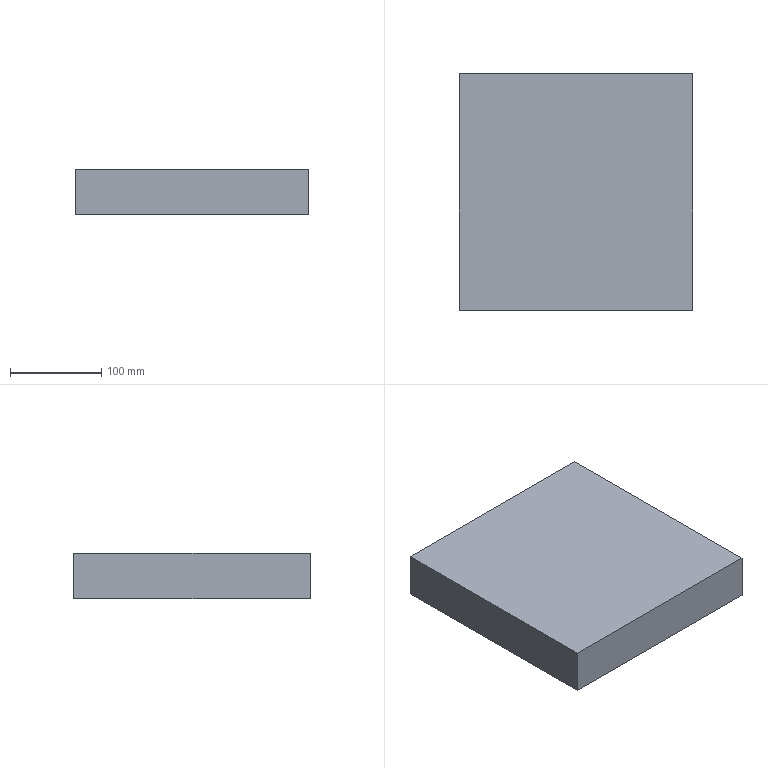Part | STEP file | 1 solid | 6 faces | box 255.311 x 259.164 x 50 mm | volume 3308367 mm3 | plane 6
STEP:
#1=CARTESIAN_POINT('',(0.,0.,0.));
#2=DIRECTION('',(0.,0.,1.));
#3=DIRECTION('',(1.,0.,0.));
#4=AXIS2_PLACEMENT_3D('',#1,#2,#3);
#5=CARTESIAN_POINT('',(-550.,-240.836,393.641));
#6=VERTEX_POINT('',#5);
#7=CARTESIAN_POINT('',(-550.,-500.,393.641));
#8=VERTEX_POINT('',#7);
#9=CARTESIAN_POINT('',(-550.,-240.836,393.641));
#10=DIRECTION('',(0.,-1.,0.));
#11=VECTOR('',#10,1.);
#12=LINE('',#9,#11);
#13=CARTESIAN_POINT('',(-550.,-240.836,343.641));
#14=DIRECTION('',(-1.,0.,0.));
#15=DIRECTION('',(0.,0.,1.));
#16=AXIS2_PLACEMENT_3D('',#13,#14,#15);
#17=PLANE('',#16);
#18=CARTESIAN_POINT('',(50.,0.));
#19=DIRECTION('',(0.,-1.));
#20=VECTOR('',#19,1.);
#21=LINE('',#18,#20);
#22=(GEOMETRIC_REPRESENTATION_CONTEXT(2)PARAMETRIC_REPRESENTATION_CONTEXT()REPRESENTATION_CONTEXT('',''));
#23=DEFINITIONAL_REPRESENTATION('',(#21),#22);
#24=PCURVE('',#17,#23);
#25=CARTESIAN_POINT('',(0.,0.,393.641));
#26=DIRECTION('',(0.,0.,1.));
#27=DIRECTION('',(1.,0.,0.));
#28=AXIS2_PLACEMENT_3D('',#25,#26,#27);
#29=PLANE('',#28);
#30=CARTESIAN_POINT('',(-550.,-240.836));
#31=DIRECTION('',(0.,-1.));
#32=VECTOR('',#31,1.);
#33=LINE('',#30,#32);
#34=(GEOMETRIC_REPRESENTATION_CONTEXT(2)PARAMETRIC_REPRESENTATION_CONTEXT()REPRESENTATION_CONTEXT('',''));
#35=DEFINITIONAL_REPRESENTATION('',(#33),#34);
#36=PCURVE('',#29,#35);
#37=SURFACE_CURVE('',#12,(#24,#36),.PCURVE_S1.);
#38=EDGE_CURVE('',#6,#8,#37,.T.);
#39=ORIENTED_EDGE('',*,*,#38,.F.);
#40=CARTESIAN_POINT('',(-550.,-240.836,343.641));
#41=VERTEX_POINT('',#40);
#42=CARTESIAN_POINT('',(-550.,-240.836,343.641));
#43=DIRECTION('',(0.,0.,1.));
#44=VECTOR('',#43,1.);
#45=LINE('',#42,#44);
#46=CARTESIAN_POINT('',(0.,0.));
#47=DIRECTION('',(1.,0.));
#48=VECTOR('',#47,1.);
#49=LINE('',#46,#48);
#50=(GEOMETRIC_REPRESENTATION_CONTEXT(2)PARAMETRIC_REPRESENTATION_CONTEXT()REPRESENTATION_CONTEXT('',''));
#51=DEFINITIONAL_REPRESENTATION('',(#49),#50);
#52=PCURVE('',#17,#51);
#53=CARTESIAN_POINT('',(-550.,-240.836,343.641));
#54=DIRECTION('',(0.,1.,0.));
#55=DIRECTION('',(0.,0.,1.));
#56=AXIS2_PLACEMENT_3D('',#53,#54,#55);
#57=PLANE('',#56);
#58=CARTESIAN_POINT('',(0.,0.));
#59=DIRECTION('',(1.,0.));
#60=VECTOR('',#59,1.);
#61=LINE('',#58,#60);
#62=(GEOMETRIC_REPRESENTATION_CONTEXT(2)PARAMETRIC_REPRESENTATION_CONTEXT()REPRESENTATION_CONTEXT('',''));
#63=DEFINITIONAL_REPRESENTATION('',(#61),#62);
#64=PCURVE('',#57,#63);
#65=SURFACE_CURVE('',#45,(#52,#64),.PCURVE_S1.);
#66=EDGE_CURVE('',#41,#6,#65,.T.);
#67=ORIENTED_EDGE('',*,*,#66,.F.);
#68=CARTESIAN_POINT('',(-550.,-500.,343.641));
#69=VERTEX_POINT('',#68);
#70=CARTESIAN_POINT('',(-550.,-240.836,343.641));
#71=DIRECTION('',(0.,-1.,0.));
#72=VECTOR('',#71,1.);
#73=LINE('',#70,#72);
#74=CARTESIAN_POINT('',(0.,0.));
#75=DIRECTION('',(0.,-1.));
#76=VECTOR('',#75,1.);
#77=LINE('',#74,#76);
#78=(GEOMETRIC_REPRESENTATION_CONTEXT(2)PARAMETRIC_REPRESENTATION_CONTEXT()REPRESENTATION_CONTEXT('',''));
#79=DEFINITIONAL_REPRESENTATION('',(#77),#78);
#80=PCURVE('',#17,#79);
#81=CARTESIAN_POINT('',(0.,0.,343.641));
#82=DIRECTION('',(0.,0.,1.));
#83=DIRECTION('',(1.,0.,0.));
#84=AXIS2_PLACEMENT_3D('',#81,#82,#83);
#85=PLANE('',#84);
#86=CARTESIAN_POINT('',(-550.,-240.836));
#87=DIRECTION('',(0.,-1.));
#88=VECTOR('',#87,1.);
#89=LINE('',#86,#88);
#90=(GEOMETRIC_REPRESENTATION_CONTEXT(2)PARAMETRIC_REPRESENTATION_CONTEXT()REPRESENTATION_CONTEXT('',''));
#91=DEFINITIONAL_REPRESENTATION('',(#89),#90);
#92=PCURVE('',#85,#91);
#93=SURFACE_CURVE('',#73,(#80,#92),.PCURVE_S1.);
#94=EDGE_CURVE('',#41,#69,#93,.T.);
#95=ORIENTED_EDGE('',*,*,#94,.T.);
#96=CARTESIAN_POINT('',(-550.,-500.,343.641));
#97=DIRECTION('',(0.,0.,1.));
#98=VECTOR('',#97,1.);
#99=LINE('',#96,#98);
#100=CARTESIAN_POINT('',(0.,-259.164));
#101=DIRECTION('',(1.,0.));
#102=VECTOR('',#101,1.);
#103=LINE('',#100,#102);
#104=(GEOMETRIC_REPRESENTATION_CONTEXT(2)PARAMETRIC_REPRESENTATION_CONTEXT()REPRESENTATION_CONTEXT('',''));
#105=DEFINITIONAL_REPRESENTATION('',(#103),#104);
#106=PCURVE('',#17,#105);
#107=CARTESIAN_POINT('',(-550.,-500.,343.641));
#108=DIRECTION('',(0.,-1.,0.));
#109=DIRECTION('',(0.,0.,-1.));
#110=AXIS2_PLACEMENT_3D('',#107,#108,#109);
#111=PLANE('',#110);
#112=CARTESIAN_POINT('',(0.,0.));
#113=DIRECTION('',(-1.,0.));
#114=VECTOR('',#113,1.);
#115=LINE('',#112,#114);
#116=(GEOMETRIC_REPRESENTATION_CONTEXT(2)PARAMETRIC_REPRESENTATION_CONTEXT()REPRESENTATION_CONTEXT('',''));
#117=DEFINITIONAL_REPRESENTATION('',(#115),#116);
#118=PCURVE('',#111,#117);
#119=SURFACE_CURVE('',#99,(#106,#118),.PCURVE_S1.);
#120=EDGE_CURVE('',#69,#8,#119,.T.);
#121=ORIENTED_EDGE('',*,*,#120,.T.);
#122=EDGE_LOOP('',(#39,#67,#95,#121));
#123=FACE_BOUND('',#122,.T.);
#124=ADVANCED_FACE('',(#123),#17,.T.);
#125=CARTESIAN_POINT('',(-294.689,-240.836,393.641));
#126=VERTEX_POINT('',#125);
#127=CARTESIAN_POINT('',(-550.,-240.836,393.641));
#128=DIRECTION('',(-1.,0.,0.));
#129=VECTOR('',#128,1.);
#130=LINE('',#127,#129);
#131=CARTESIAN_POINT('',(50.,0.));
#132=DIRECTION('',(0.,-1.));
#133=VECTOR('',#132,1.);
#134=LINE('',#131,#133);
#135=(GEOMETRIC_REPRESENTATION_CONTEXT(2)PARAMETRIC_REPRESENTATION_CONTEXT()REPRESENTATION_CONTEXT('',''));
#136=DEFINITIONAL_REPRESENTATION('',(#134),#135);
#137=PCURVE('',#57,#136);
#138=CARTESIAN_POINT('',(-550.,-240.836));
#139=DIRECTION('',(-1.,0.));
#140=VECTOR('',#139,1.);
#141=LINE('',#138,#140);
#142=(GEOMETRIC_REPRESENTATION_CONTEXT(2)PARAMETRIC_REPRESENTATION_CONTEXT()REPRESENTATION_CONTEXT('',''));
#143=DEFINITIONAL_REPRESENTATION('',(#141),#142);
#144=PCURVE('',#29,#143);
#145=SURFACE_CURVE('',#130,(#137,#144),.PCURVE_S1.);
#146=EDGE_CURVE('',#126,#6,#145,.T.);
#147=ORIENTED_EDGE('',*,*,#146,.F.);
#148=CARTESIAN_POINT('',(-294.689,-240.836,343.641));
#149=VERTEX_POINT('',#148);
#150=CARTESIAN_POINT('',(-294.689,-240.836,343.641));
#151=DIRECTION('',(0.,0.,1.));
#152=VECTOR('',#151,1.);
#153=LINE('',#150,#152);
#154=CARTESIAN_POINT('',(0.,255.311));
#155=DIRECTION('',(1.,0.));
#156=VECTOR('',#155,1.);
#157=LINE('',#154,#156);
#158=(GEOMETRIC_REPRESENTATION_CONTEXT(2)PARAMETRIC_REPRESENTATION_CONTEXT()REPRESENTATION_CONTEXT('',''));
#159=DEFINITIONAL_REPRESENTATION('',(#157),#158);
#160=PCURVE('',#57,#159);
#161=CARTESIAN_POINT('',(-294.689,-240.836,343.641));
#162=DIRECTION('',(1.,0.,0.));
#163=DIRECTION('',(0.,0.,-1.));
#164=AXIS2_PLACEMENT_3D('',#161,#162,#163);
#165=PLANE('',#164);
#166=CARTESIAN_POINT('',(0.,0.));
#167=DIRECTION('',(-1.,0.));
#168=VECTOR('',#167,1.);
#169=LINE('',#166,#168);
#170=(GEOMETRIC_REPRESENTATION_CONTEXT(2)PARAMETRIC_REPRESENTATION_CONTEXT()REPRESENTATION_CONTEXT('',''));
#171=DEFINITIONAL_REPRESENTATION('',(#169),#170);
#172=PCURVE('',#165,#171);
#173=SURFACE_CURVE('',#153,(#160,#172),.PCURVE_S1.);
#174=EDGE_CURVE('',#149,#126,#173,.T.);
#175=ORIENTED_EDGE('',*,*,#174,.F.);
#176=CARTESIAN_POINT('',(-550.,-240.836,343.641));
#177=DIRECTION('',(-1.,0.,0.));
#178=VECTOR('',#177,1.);
#179=LINE('',#176,#178);
#180=CARTESIAN_POINT('',(0.,0.));
#181=DIRECTION('',(0.,-1.));
#182=VECTOR('',#181,1.);
#183=LINE('',#180,#182);
#184=(GEOMETRIC_REPRESENTATION_CONTEXT(2)PARAMETRIC_REPRESENTATION_CONTEXT()REPRESENTATION_CONTEXT('',''));
#185=DEFINITIONAL_REPRESENTATION('',(#183),#184);
#186=PCURVE('',#57,#185);
#187=CARTESIAN_POINT('',(-550.,-240.836));
#188=DIRECTION('',(-1.,0.));
#189=VECTOR('',#188,1.);
#190=LINE('',#187,#189);
#191=(GEOMETRIC_REPRESENTATION_CONTEXT(2)PARAMETRIC_REPRESENTATION_CONTEXT()REPRESENTATION_CONTEXT('',''));
#192=DEFINITIONAL_REPRESENTATION('',(#190),#191);
#193=PCURVE('',#85,#192);
#194=SURFACE_CURVE('',#179,(#186,#193),.PCURVE_S1.);
#195=EDGE_CURVE('',#149,#41,#194,.T.);
#196=ORIENTED_EDGE('',*,*,#195,.T.);
#197=ORIENTED_EDGE('',*,*,#66,.T.);
#198=EDGE_LOOP('',(#147,#175,#196,#197));
#199=FACE_BOUND('',#198,.T.);
#200=ADVANCED_FACE('',(#199),#57,.T.);
#201=CARTESIAN_POINT('',(-294.689,-500.,393.641));
#202=VERTEX_POINT('',#201);
#203=CARTESIAN_POINT('',(-294.689,-240.836,393.641));
#204=DIRECTION('',(0.,1.,0.));
#205=VECTOR('',#204,1.);
#206=LINE('',#203,#205);
#207=CARTESIAN_POINT('',(-50.,0.));
#208=DIRECTION('',(0.,1.));
#209=VECTOR('',#208,1.);
#210=LINE('',#207,#209);
#211=(GEOMETRIC_REPRESENTATION_CONTEXT(2)PARAMETRIC_REPRESENTATION_CONTEXT()REPRESENTATION_CONTEXT('',''));
#212=DEFINITIONAL_REPRESENTATION('',(#210),#211);
#213=PCURVE('',#165,#212);
#214=CARTESIAN_POINT('',(-294.689,-240.836));
#215=DIRECTION('',(0.,1.));
#216=VECTOR('',#215,1.);
#217=LINE('',#214,#216);
#218=(GEOMETRIC_REPRESENTATION_CONTEXT(2)PARAMETRIC_REPRESENTATION_CONTEXT()REPRESENTATION_CONTEXT('',''));
#219=DEFINITIONAL_REPRESENTATION('',(#217),#218);
#220=PCURVE('',#29,#219);
#221=SURFACE_CURVE('',#206,(#213,#220),.PCURVE_S1.);
#222=EDGE_CURVE('',#202,#126,#221,.T.);
#223=ORIENTED_EDGE('',*,*,#222,.F.);
#224=CARTESIAN_POINT('',(-294.689,-500.,343.641));
#225=VERTEX_POINT('',#224);
#226=CARTESIAN_POINT('',(-294.689,-500.,343.641));
#227=DIRECTION('',(0.,0.,1.));
#228=VECTOR('',#227,1.);
#229=LINE('',#226,#228);
#230=CARTESIAN_POINT('',(0.,-259.164));
#231=DIRECTION('',(-1.,0.));
#232=VECTOR('',#231,1.);
#233=LINE('',#230,#232);
#234=(GEOMETRIC_REPRESENTATION_CONTEXT(2)PARAMETRIC_REPRESENTATION_CONTEXT()REPRESENTATION_CONTEXT('',''));
#235=DEFINITIONAL_REPRESENTATION('',(#233),#234);
#236=PCURVE('',#165,#235);
#237=CARTESIAN_POINT('',(0.,255.311));
#238=DIRECTION('',(-1.,0.));
#239=VECTOR('',#238,1.);
#240=LINE('',#237,#239);
#241=(GEOMETRIC_REPRESENTATION_CONTEXT(2)PARAMETRIC_REPRESENTATION_CONTEXT()REPRESENTATION_CONTEXT('',''));
#242=DEFINITIONAL_REPRESENTATION('',(#240),#241);
#243=PCURVE('',#111,#242);
#244=SURFACE_CURVE('',#229,(#236,#243),.PCURVE_S1.);
#245=EDGE_CURVE('',#225,#202,#244,.T.);
#246=ORIENTED_EDGE('',*,*,#245,.F.);
#247=CARTESIAN_POINT('',(-294.689,-240.836,343.641));
#248=DIRECTION('',(0.,1.,0.));
#249=VECTOR('',#248,1.);
#250=LINE('',#247,#249);
#251=CARTESIAN_POINT('',(0.,0.));
#252=DIRECTION('',(0.,1.));
#253=VECTOR('',#252,1.);
#254=LINE('',#251,#253);
#255=(GEOMETRIC_REPRESENTATION_CONTEXT(2)PARAMETRIC_REPRESENTATION_CONTEXT()REPRESENTATION_CONTEXT('',''));
#256=DEFINITIONAL_REPRESENTATION('',(#254),#255);
#257=PCURVE('',#165,#256);
#258=CARTESIAN_POINT('',(-294.689,-240.836));
#259=DIRECTION('',(0.,1.));
#260=VECTOR('',#259,1.);
#261=LINE('',#258,#260);
#262=(GEOMETRIC_REPRESENTATION_CONTEXT(2)PARAMETRIC_REPRESENTATION_CONTEXT()REPRESENTATION_CONTEXT('',''));
#263=DEFINITIONAL_REPRESENTATION('',(#261),#262);
#264=PCURVE('',#85,#263);
#265=SURFACE_CURVE('',#250,(#257,#264),.PCURVE_S1.);
#266=EDGE_CURVE('',#225,#149,#265,.T.);
#267=ORIENTED_EDGE('',*,*,#266,.T.);
#268=ORIENTED_EDGE('',*,*,#174,.T.);
#269=EDGE_LOOP('',(#223,#246,#267,#268));
#270=FACE_BOUND('',#269,.T.);
#271=ADVANCED_FACE('',(#270),#165,.T.);
#272=CARTESIAN_POINT('',(-550.,-500.,393.641));
#273=DIRECTION('',(1.,0.,0.));
#274=VECTOR('',#273,1.);
#275=LINE('',#272,#274);
#276=CARTESIAN_POINT('',(-50.,0.));
#277=DIRECTION('',(0.,1.));
#278=VECTOR('',#277,1.);
#279=LINE('',#276,#278);
#280=(GEOMETRIC_REPRESENTATION_CONTEXT(2)PARAMETRIC_REPRESENTATION_CONTEXT()REPRESENTATION_CONTEXT('',''));
#281=DEFINITIONAL_REPRESENTATION('',(#279),#280);
#282=PCURVE('',#111,#281);
#283=CARTESIAN_POINT('',(-550.,-500.));
#284=DIRECTION('',(1.,0.));
#285=VECTOR('',#284,1.);
#286=LINE('',#283,#285);
#287=(GEOMETRIC_REPRESENTATION_CONTEXT(2)PARAMETRIC_REPRESENTATION_CONTEXT()REPRESENTATION_CONTEXT('',''));
#288=DEFINITIONAL_REPRESENTATION('',(#286),#287);
#289=PCURVE('',#29,#288);
#290=SURFACE_CURVE('',#275,(#282,#289),.PCURVE_S1.);
#291=EDGE_CURVE('',#8,#202,#290,.T.);
#292=ORIENTED_EDGE('',*,*,#291,.F.);
#293=ORIENTED_EDGE('',*,*,#120,.F.);
#294=CARTESIAN_POINT('',(-550.,-500.,343.641));
#295=DIRECTION('',(1.,0.,0.));
#296=VECTOR('',#295,1.);
#297=LINE('',#294,#296);
#298=CARTESIAN_POINT('',(0.,0.));
#299=DIRECTION('',(0.,1.));
#300=VECTOR('',#299,1.);
#301=LINE('',#298,#300);
#302=(GEOMETRIC_REPRESENTATION_CONTEXT(2)PARAMETRIC_REPRESENTATION_CONTEXT()REPRESENTATION_CONTEXT('',''));
#303=DEFINITIONAL_REPRESENTATION('',(#301),#302);
#304=PCURVE('',#111,#303);
#305=CARTESIAN_POINT('',(-550.,-500.));
#306=DIRECTION('',(1.,0.));
#307=VECTOR('',#306,1.);
#308=LINE('',#305,#307);
#309=(GEOMETRIC_REPRESENTATION_CONTEXT(2)PARAMETRIC_REPRESENTATION_CONTEXT()REPRESENTATION_CONTEXT('',''));
#310=DEFINITIONAL_REPRESENTATION('',(#308),#309);
#311=PCURVE('',#85,#310);
#312=SURFACE_CURVE('',#297,(#304,#311),.PCURVE_S1.);
#313=EDGE_CURVE('',#69,#225,#312,.T.);
#314=ORIENTED_EDGE('',*,*,#313,.T.);
#315=ORIENTED_EDGE('',*,*,#245,.T.);
#316=EDGE_LOOP('',(#292,#293,#314,#315));
#317=FACE_BOUND('',#316,.T.);
#318=ADVANCED_FACE('',(#317),#111,.T.);
#319=ORIENTED_EDGE('',*,*,#94,.F.);
#320=ORIENTED_EDGE('',*,*,#195,.F.);
#321=ORIENTED_EDGE('',*,*,#266,.F.);
#322=ORIENTED_EDGE('',*,*,#313,.F.);
#323=EDGE_LOOP('',(#319,#320,#321,#322));
#324=FACE_BOUND('',#323,.T.);
#325=ADVANCED_FACE('',(#324),#85,.F.);
#326=ORIENTED_EDGE('',*,*,#38,.T.);
#327=ORIENTED_EDGE('',*,*,#291,.T.);
#328=ORIENTED_EDGE('',*,*,#222,.T.);
#329=ORIENTED_EDGE('',*,*,#146,.T.);
#330=EDGE_LOOP('',(#326,#327,#328,#329));
#331=FACE_BOUND('',#330,.T.);
#332=ADVANCED_FACE('',(#331),#29,.T.);
#333=CLOSED_SHELL('',(#124,#200,#271,#318,#325,#332));
#334=MANIFOLD_SOLID_BREP('',#333);
#335=(LENGTH_UNIT()NAMED_UNIT(*)SI_UNIT(.MILLI.,.METRE.));
#336=UNCERTAINTY_MEASURE_WITH_UNIT(LENGTH_MEASURE(0.0000001),#335,'','');
#337=(NAMED_UNIT(*)PLANE_ANGLE_UNIT()SI_UNIT($,.RADIAN.));
#338=(NAMED_UNIT(*)SI_UNIT($,.STERADIAN.)SOLID_ANGLE_UNIT());
#339=(GEOMETRIC_REPRESENTATION_CONTEXT(3)GLOBAL_UNCERTAINTY_ASSIGNED_CONTEXT((#336))GLOBAL_UNIT_ASSIGNED_CONTEXT((#335,#337,#338))REPRESENTATION_CONTEXT('',''));
#340=ADVANCED_BREP_SHAPE_REPRESENTATION('',(#4,#334),#339);